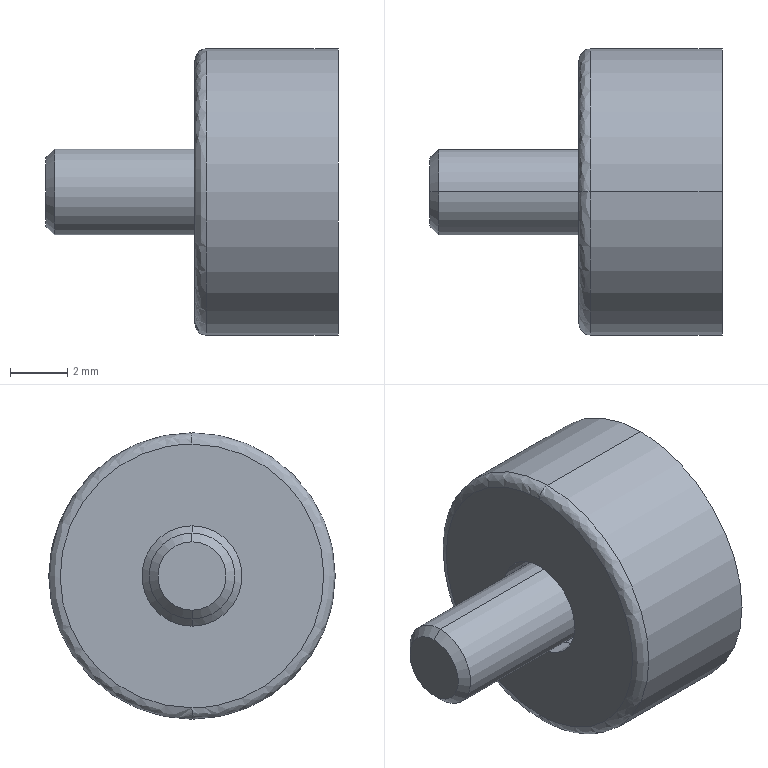Part | STEP file | BMF01-A10 Yihe Da Magnet-dddeger | 3 solids | 43 faces | box 10.2 x 10 x 10 mm | volume 381.53 mm3 | plane 19 | cylinder 14 | cone 8 | spline 2 | commonest cylinder face diameters 3.5 x4 3 x2 6 x2 8 x2 8.4 x2 10 x2